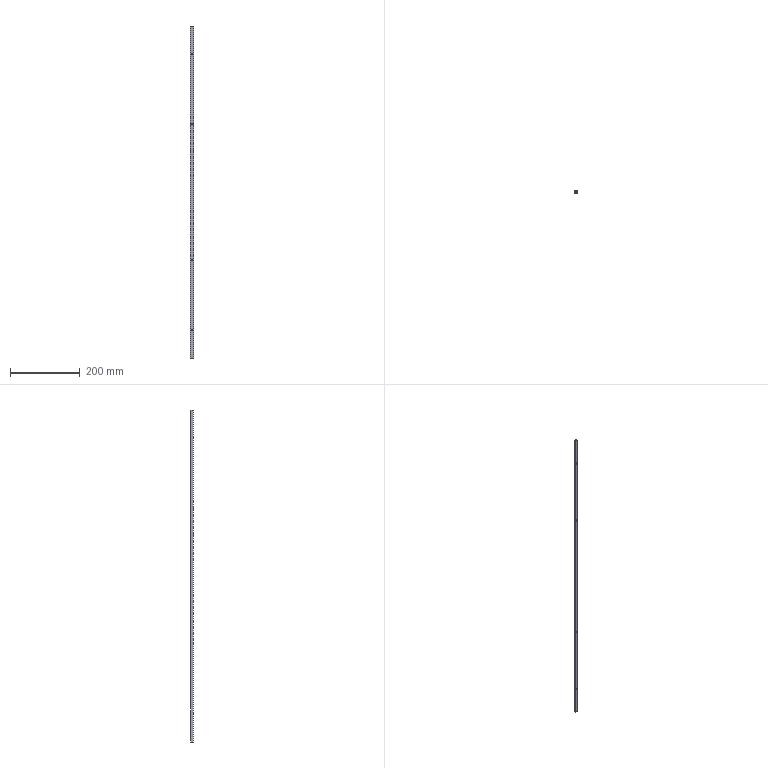Part | STEP file | 9x6 sensor aluminium slot M3 type-L950 | 1 solid | 58 faces | box 9 x 6 x 950 mm | volume 30935 mm3 | plane 42 | cone 8 | cylinder 8 | commonest cylinder face diameters 6.6 x8